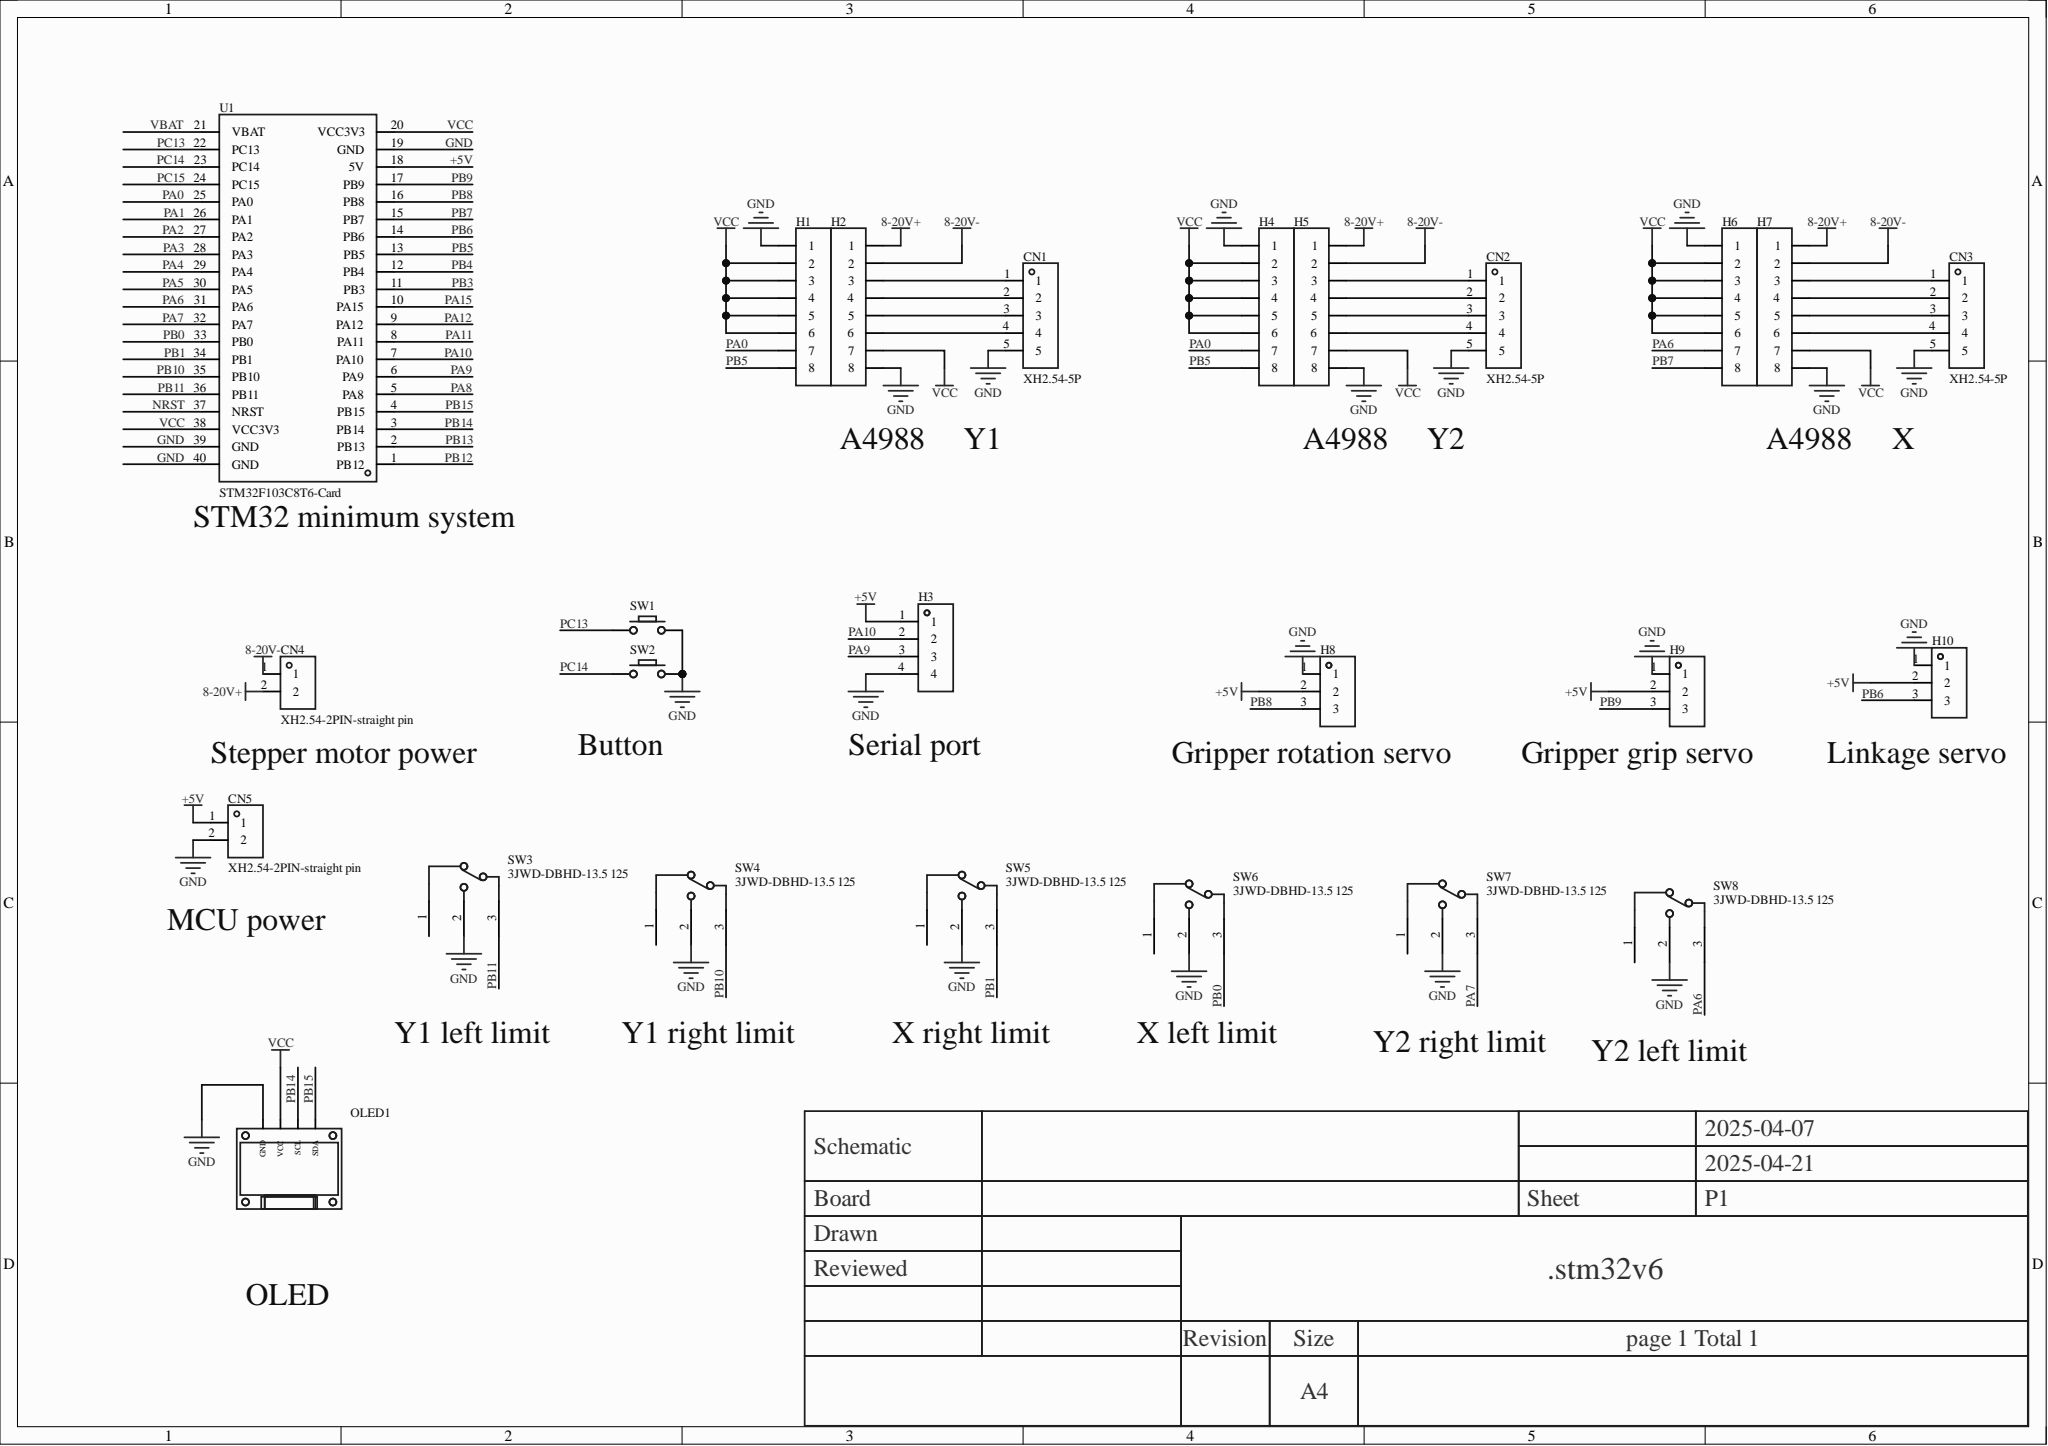Circuit board | Altium Designer | 25 parts | 35 nets
Bill of materials:
Comment,Description,Designator,Footprint,LibRef,Quantity
"XH2.54-5P","","CN1, CN2, CN3","CONN-TH_5P-P2.54_C9900008095","XH2.54-5P","3"
"XH2.54-2PIN-straight pin","","CN4, CN5","CONN-TH_XH2.54-2P","XH2.54-2PIN-直针","2"
"","","H1, H2, H4, H5, H6, H7","HDR-TH_8P-P2.54-V-F-1","HDR-F_2.54_1x8P","6"
"","","H3","HDR-TH_4P-P2.54-V-F","HDR-F_2.54_1x4P","1"
"","","H8, H9, H10","HDR-TH_3P-P2.54-V-F","HDR-F_2.54_1x3P","3"
"","","OLED1","0.96OLED_4P","0.96OLED模块_4P","1"
"","","SW1, SW2","Key_TH_3.5x6x4.3","Key_TH_3.5x6x4.3","2"
"3JWD-DBHD-13.5 125","Circuit structure: SPDT; rated current (DC): 50mA; rated voltage (DC): 125V; rated current (AC): -; rated voltage (AC): -; operating life: 5万 cycles;","SW3, SW4, SW5, SW6, SW7, SW8","SW-TH_SHOU-HAN_3JWD-DBHD-13.5","3JWD-DBHD-13.5 125","6"
"STM32F103C8T6-Card","","U1","CONN-TH_L53.3-W22.9_STM32F103C8T6-CARD","STM32F103C8T6-Card","1"
Netlist (Protel format):
[
CN1
CONN-TH_5P-P2.54_C9900008095
XH2.54-5P



]
[
CN2
CONN-TH_5P-P2.54_C9900008095
XH2.54-5P



]
[
CN3
CONN-TH_5P-P2.54_C9900008095
XH2.54-5P



]
[
CN4
CONN-TH_XH2.54-2P
XH2.54-2PIN-straight pin



]
[
CN5
CONN-TH_XH2.54-2P
XH2.54-2PIN-straight pin



]
[
H1
HDR-TH_8P-P2.54-V-F-1




]
[
H2
HDR-TH_8P-P2.54-V-F-1




]
[
H3
HDR-TH_4P-P2.54-V-F




]
[
H4
HDR-TH_8P-P2.54-V-F-1




]
[
H5
HDR-TH_8P-P2.54-V-F-1




]
[
H6
HDR-TH_8P-P2.54-V-F-1




]
[
H7
HDR-TH_8P-P2.54-V-F-1




]
[
H8
HDR-TH_3P-P2.54-V-F




]
[
H9
HDR-TH_3P-P2.54-V-F




]
[
H10
HDR-TH_3P-P2.54-V-F




]
[
OLED1
0.96OLED_4P




]
[
SW1
Key_TH_3.5x6x4.3




]
[
SW2
Key_TH_3.5x6x4.3




]
[
SW3
SW-TH_SHOU-HAN_3JWD-DBHD-13.5
3JWD-DBHD-13.5 125



]
[
SW4
SW-TH_SHOU-HAN_3JWD-DBHD-13.5
3JWD-DBHD-13.5 125



]
[
SW5
SW-TH_SHOU-HAN_3JWD-DBHD-13.5
3JWD-DBHD-13.5 125



]
[
SW6
SW-TH_SHOU-HAN_3JWD-DBHD-13.5
3JWD-DBHD-13.5 125



]
[
SW7
SW-TH_SHOU-HAN_3JWD-DBHD-13.5
3JWD-DBHD-13.5 125



]
[
SW8
SW-TH_SHOU-HAN_3JWD-DBHD-13.5
3JWD-DBHD-13.5 125



]
[
U1
CONN-TH_L53.3-W22.9_STM32F103C8T6-CARD
STM32F103C8T6-Card



]
(
VCC
H1-2
H1-3
H1-4
H1-5
H1-6
H2-7
H4-2
H4-3
H4-4
H4-5
H4-6
H5-7
H6-2
H6-3
H6-4
H6-5
H6-6
H7-7
OLED1-2
U1-20
U1-38
)
(
PC14
SW2-A
U1-23
)
(
PC13
SW1-A
U1-22
)
(
PB15
OLED1-4
U1-4
)
(
PB14
OLED1-3
U1-3
)
(
PB11
SW3-3
U1-36
)
(
PB10
SW4-3
U1-35
)
(
PB9
H9-3
U1-17
)
(
PB8
H8-3
U1-16
)
(
PB7
H6-8
U1-15
)
(
PB6
H10-3
U1-14
)
(
PB5
H1-8
H4-8
U1-13
)
(
PB1
SW5-3
U1-34
)
(
PB0
SW6-3
U1-33
)
(
PA10
H3-2
U1-7
)
(
PA9
H3-3
U1-6
)
(
PA7
SW7-3
U1-32
)
(
PA6
H6-7
SW8-3
U1-31
)
(
PA0
H1-7
H4-7
U1-25
)
(
NetCN3_4
CN3-4
H7-6
)
(
NetCN3_3
CN3-3
H7-5
)
(
NetCN3_2
CN3-2
H7-4
)
(
NetCN3_1
CN3-1
H7-3
)
(
NetCN2_4
CN2-4
H5-6
)
(
NetCN2_3
CN2-3
H5-5
)
(
NetCN2_2
CN2-2
H5-4
)
(
NetCN2_1
CN2-1
H5-3
)
(
NetCN1_4
CN1-4
H2-6
)
(
NetCN1_3
CN1-3
H2-5
)
(
NetCN1_2
CN1-2
H2-4
)
(
NetCN1_1
CN1-1
H2-3
)
(
GND
CN1-5
CN2-5
CN3-5
CN5-2
H1-1
H2-8
H3-4
H4-1
H5-8
H6-1
H7-8
H8-1
H9-1
H10-1
OLED1-1
SW1-B
SW2-B
SW3-2
SW4-2
SW5-2
SW6-2
SW7-2
SW8-2
U1-19
U1-39
U1-40
)
(
+5V
CN5-1
H3-1
H8-2
H9-2
H10-2
U1-18
)
(
8-20V-
CN4-1
H2-2
H5-2
H7-2
)
(
8-20V+
CN4-2
H2-1
H5-1
H7-1
)